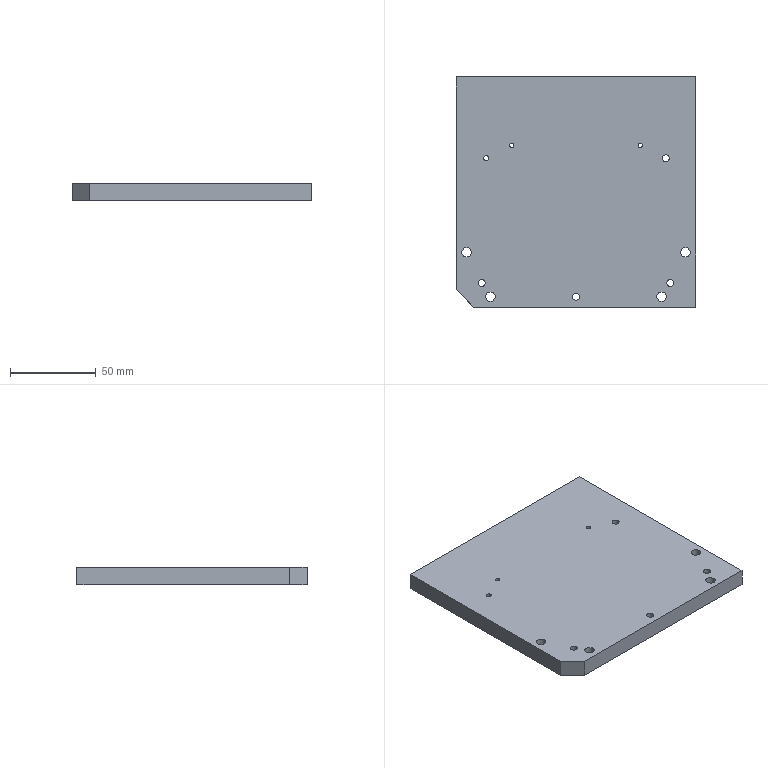CAM job | NX | 3-axis milling, drilling | part box 140 x 134.5 x 10 mm | stock box 145 x 140 x 12 mm
Tools:
number,name,description,diameter,corner_radius,flute_length,length,flutes
6,D6,平底铣刀-粗,6.0,0.0,25.0,75.0,2
9,D10,平底铣刀-粗,10.0,0.0,35.0,75.0,2
7,D6-J,平底铣刀-精,6.0,0.0,25.0,75.0,2
1,D80R0.8_FLYCUTTER,圆鼻刀-粗,80.0,0.8,50.0,75.0,2
1,D80R0.8_FLYCUTTER-J,圆鼻刀-精,80.0,0.8,50.0,75.0,2
2,D6_CHAMFERMILL,倒角刀,6.0,0.0,3.0,25.0,2
20,M3X0.5,丝锥,2.5,0.0,35.0,50.0,2
22,D3_REAMER,Drilling Tool,3.0,0.0,75.0,100.0,6
23,D4_REAMER,Drilling Tool,4.0,0.0,75.0,100.0,6
12,ZT2.6,钻头,2.6,0.0,35.0,50.0,2
19,ZT5.5,钻头,5.5,0.0,35.0,50.0,2
17,ZT2.9,Drilling Tool,2.9,0.0,35.0,50.0,2
18,ZT3.9,Drilling Tool,3.9,0.0,35.0,50.0,2
Operations:
program,operation,operation_type,tool,method,geometry_group,spindle_rpm,surface_speed,feed_per_tooth,feed_cut,feed_plunge,cut_length_mm,path_length_mm,cut_time_min,machine_time_min
B,FLOORWALLFLYROUGH_COPY,VolumeBased25DMillingOperation,D80R0.8_FLYCUTTER,LAYERROUGH-DEPTHK-STEPG,W-B,2800.0,703.696,0.5357,3000.0,100.0,3019.47,3884.12,1.006,1.093
B,FLOORWALLFLYFINISH_COPY,VolumeBased25DMillingOperation,D80R0.8_FLYCUTTER-J,SIDEFINISH-DEPTHK-STEPG,W-B,4000.0,1005.28,0.125,1000.0,100.0,754.084,850.084,0.7541,0.7637
B,NG_DRILLCHAMFER_4,Operation,D6_CHAMFERMILL,METHOD,W-B,8000.0,150.796,0.0625,1000.0,0.0,9.5,197.06,0.0095,0.0283
B,NG_DRILLCHAMFER_5,Operation,D6_CHAMFERMILL,METHOD,W-B,8000.0,150.796,0.0625,1000.0,0.0,4.8,109.6,0.0048,0.0153
B,NG_DRILLCHAMFER_6,Operation,D6_CHAMFERMILL,METHOD,W-B,8000.0,150.796,0.0625,1000.0,0.0,21.2,335.824,0.0212,0.0527
B,MILLCHAMFER_3,PlanarMilling,D6_CHAMFERMILL,METHOD,W-B,8000.0,150.796,0.075,1200.0,100.0,71.178,637.459,0.0593,0.1159
B,PLANARDEBURR6X45L_COPY,SurfaceContour,D6_CHAMFERMILL,SLOPECHAMFER-DEPTH0-STEPG,W-B,6500.0,122.519,0.1154,1500.0,100.0,660.793,1248.395,0.4405,0.4993
A,TOPFACE,FaceMilling,D80R0.8_FLYCUTTER,SIDEFINISH-DEPTHK-STEPG,W-A,4500.0,1385.0,0.1667,1500.0,100.0,781.25,877.25,0.5208,0.5304
A,OUTLINEROUGH_2,VolumeBased25DMillingOperation,D10,METHOD,W-A,8000.0,251.327,0.375,6000.0,80.0,8629.302,8737.802,1.438,1.449
A,STEPROUGH_2,CavityMilling,D10,METHOD,W-A,9000.0,282.743,0.1944,3500.0,100.0,4178.844,4571.202,1.224,1.263
A,FLOORWALLROUGH_1,VolumeBased25DMillingOperation,D10,METHOD,W-A,9000.0,169.646,0.2778,5000.0,100.0,1161.182,3399.482,0.2322,0.4561
A,SPOTDRILL-DEPTH0.8,Operation,D6_CHAMFERMILL,NONE,W-A,8000.0,150.796,0.0312,500.0,90.0,19.8,454.89,0.0396,0.0831
A,SPOTDRILL-DEPTH0.8_2,Operation,D6_CHAMFERMILL,NONE,W-A,8000.0,150.796,0.0312,500.0,90.0,3.6,183.207,0.0072,0.0252
A,THRUHOLE-M3TAPDRILL,Operation,ZT2.6,NONE,W-A,3000.0,23.562,0.05,300.0,90.0,34.0,244.007,0.1133,0.1343
A,THRUHOLE-FINISHHOLE3.0PREDRILL,Operation,ZT2.9,NONE,W-A,3200.0,29.154,0.0312,200.0,90.0,14.837,129.674,0.0742,0.0857
A,THRUHOLE-FINISHHOLE4.0PREDRILL,Operation,ZT3.9,NONE,W-A,3000.0,36.757,0.0417,250.0,90.0,60.503,408.232,0.242,0.2768
A,COUNTERBORE-DRILL0SEG,Operation,ZT5.5,NONE,W-A,1200.0,20.735,0.0625,150.0,90.0,58.609,379.317,0.3907,0.4228
A,HOLEROUGHD6_1,CylinderMilling,D6,NONE,W-A,8000.0,150.796,0.075,1200.0,100.0,635.598,1214.258,0.5297,0.5875
A,HOLEROUGHD6_2,CylinderMilling,D6,NONE,W-A,8000.0,150.796,0.075,1200.0,100.0,232.955,513.955,0.1941,0.2222
A,HOLEFINISHD6_1,CylinderMilling,D6-J,FINISHSTEPDEPTHOFF,W-A,8000.0,150.796,0.0312,500.0,100.0,133.594,714.254,0.2672,0.3253
A,HOLEFINISHD6_2,CylinderMilling,D6-J,FINISHSTEPDEPTHOFF,W-A,8000.0,150.796,0.0312,500.0,100.0,57.873,339.873,0.1157,0.1439
A,BOTTOMFINISH_1,VolumeBased25DMillingOperation,D6-J,METHOD,W-A,8000.0,150.796,0.075,1200.0,100.0,443.062,555.062,0.3692,0.3804
A,FLOORWALLFINISHBOTTOM-MID_COPY,VolumeBased25DMillingOperation,D6-J,FINISHSTEPDEPTHOFF,W-A,7000.0,175.0,0.0536,1500.0,100.0,274.442,306.242,0.183,0.1861
A,BOTTOMSIDEFINISH_3,VolumeBased25DMillingOperation,D6-J,METHOD,W-A,8000.0,150.796,0.075,1200.0,100.0,167.408,280.398,0.1395,0.1508
A,BOTTOMSIDEFINISH_4,VolumeBased25DMillingOperation,D6-J,METHOD,W-A,9000.0,169.646,0.0833,1500.0,100.0,86.025,199.025,0.0573,0.0686
A,SOLIDONLY,SurfaceContour,D6_CHAMFERMILL,METHOD,W-A,8000.0,150.796,0.1875,3000.0,100.0,844.449,1290.991,0.2815,0.3261
A,NG_DRILLCHAMFER_1,Operation,D6_CHAMFERMILL,METHOD,W-A,8000.0,150.796,0.0312,500.0,0.0,4.8,109.6,0.0096,0.0201
A,NG_DRILLCHAMFER_2,Operation,D6_CHAMFERMILL,METHOD,W-A,8000.0,150.796,0.0312,500.0,0.0,21.2,335.824,0.0424,0.0739
A,MILLCHAMFER_1,PlanarMilling,D6_CHAMFERMILL,NONE,W-A,8000.0,150.796,0.05,800.0,100.0,161.004,692.09,0.2013,0.2544
A,MILLCHAMFER_2,PlanarMilling,D6_CHAMFERMILL,NONE,W-A,8000.0,150.796,0.05,800.0,100.0,81.13,355.143,0.1014,0.1288
A,NG_DRILLCHAMFER_3,Operation,D6_CHAMFERMILL,METHOD,W-A,8000.0,150.796,0.0312,500.0,0.0,17.1,212.26,0.0342,0.0537
A,REAMING,Operation,D3_REAMER,METHOD,W-A,500.0,4.712,0.0167,50.0,0.0,12.0,124.0,0.24,0.2512
A,REAMING_2,Operation,D4_REAMER,METHOD,W-A,500.0,6.283,0.0167,50.0,0.0,48.0,383.225,0.96,0.9935
A,THRUHOLE-TAPM3,Operation,M3X0.5,METHOD,W-A,800.0,6.283,0.0003,0.5,90.0,28.0,232.007,56.0,56.02
A,OUTLINESEMI_2,VolumeBased25DMillingOperation,D6-J,METHOD,W-A,9000.0,169.646,0.0667,1200.0,100.0,566.908,685.908,0.4724,0.4843